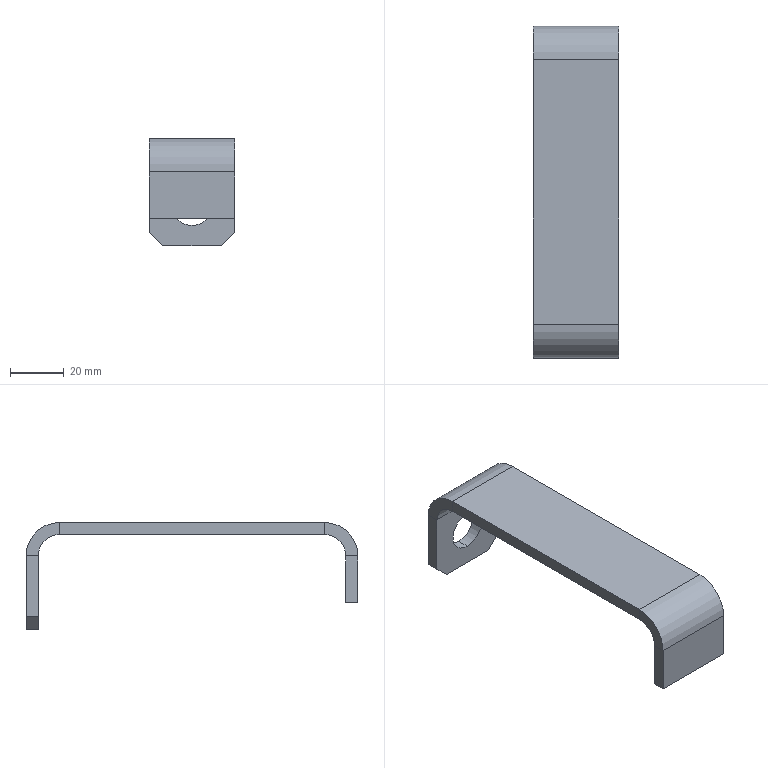Part | SolidWorks | features Chamfer 1, FlatPattern 1, ICE 1, SMBaseFlange 1, SheetMetal 1 | 1 solid | 26 faces | box 32 x 124 x 40 mm | volume 24465 mm3 | plane 20 | cylinder 6 | commonest cylinder face diameters 15 x2 16 x2 25 x2
STEP:
#1=CARTESIAN_POINT('',(0.,119.5,12.5));
#2=VERTEX_POINT('',#1);
#3=CARTESIAN_POINT('',(0.,119.5,-2.5));
#4=VERTEX_POINT('',#3);
#5=CARTESIAN_POINT('',(0.,119.5,5.));
#6=DIRECTION('',(0.,-1.,0.));
#7=DIRECTION('',(0.,0.,1.));
#8=AXIS2_PLACEMENT_3D('',#5,#6,#7);
#9=CIRCLE('',#8,7.5);
#10=EDGE_CURVE('',#2,#4,#9,.T.);
#11=ORIENTED_EDGE('',*,*,#10,.T.);
#12=CARTESIAN_POINT('',(0.,124.,-2.5));
#13=VERTEX_POINT('',#12);
#14=CARTESIAN_POINT('',(0.,-0.001,-2.5));
#15=DIRECTION('',(0.,1.,0.));
#16=VECTOR('',#15,1000.);
#17=LINE('',#14,#16);
#18=EDGE_CURVE('',#4,#13,#17,.T.);
#19=ORIENTED_EDGE('',*,*,#18,.T.);
#20=CARTESIAN_POINT('',(0.,124.,12.5));
#21=VERTEX_POINT('',#20);
#22=CARTESIAN_POINT('',(0.,124.,5.));
#23=DIRECTION('',(0.,1.,0.));
#24=DIRECTION('',(0.,0.,1.));
#25=AXIS2_PLACEMENT_3D('',#22,#23,#24);
#26=CIRCLE('',#25,7.5);
#27=EDGE_CURVE('',#13,#21,#26,.T.);
#28=ORIENTED_EDGE('',*,*,#27,.T.);
#29=CARTESIAN_POINT('',(0.,-0.001,12.5));
#30=DIRECTION('',(0.,1.,0.));
#31=VECTOR('',#30,1000.);
#32=LINE('',#29,#31);
#33=EDGE_CURVE('',#2,#21,#32,.T.);
#34=ORIENTED_EDGE('',*,*,#33,.F.);
#35=EDGE_LOOP('',(#11,#19,#28,#34));
#36=FACE_OUTER_BOUND('',#35,.T.);
#37=CARTESIAN_POINT('',(0.,-0.001,5.));
#38=DIRECTION('',(0.,1.,0.));
#39=DIRECTION('',(0.,0.,1.));
#40=AXIS2_PLACEMENT_3D('',#37,#38,#39);
#41=CYLINDRICAL_SURFACE('',#40,7.5);
#42=ADVANCED_FACE('',(#36),#41,.F.);
#43=CARTESIAN_POINT('',(16.,12.5,30.));
#44=VERTEX_POINT('',#43);
#45=CARTESIAN_POINT('',(16.,12.5,25.5));
#46=VERTEX_POINT('',#45);
#47=CARTESIAN_POINT('',(16.,12.5,30.));
#48=DIRECTION('',(0.,0.,-1.));
#49=VECTOR('',#48,1000.);
#50=LINE('',#47,#49);
#51=EDGE_CURVE('',#44,#46,#50,.T.);
#52=ORIENTED_EDGE('',*,*,#51,.F.);
#53=CARTESIAN_POINT('',(16.,0.,17.5));
#54=VERTEX_POINT('',#53);
#55=CARTESIAN_POINT('',(16.,12.5,17.5));
#56=DIRECTION('',(-1.,0.,0.));
#57=DIRECTION('',(0.,0.,-1.));
#58=AXIS2_PLACEMENT_3D('',#55,#56,#57);
#59=CIRCLE('',#58,12.5);
#60=EDGE_CURVE('',#54,#44,#59,.T.);
#61=ORIENTED_EDGE('',*,*,#60,.F.);
#62=CARTESIAN_POINT('',(16.,4.5,17.5));
#63=VERTEX_POINT('',#62);
#64=CARTESIAN_POINT('',(16.,4.5,17.5));
#65=DIRECTION('',(0.,-1.,0.));
#66=VECTOR('',#65,1000.);
#67=LINE('',#64,#66);
#68=EDGE_CURVE('',#63,#54,#67,.T.);
#69=ORIENTED_EDGE('',*,*,#68,.F.);
#70=CARTESIAN_POINT('',(16.,12.5,17.5));
#71=DIRECTION('',(-1.,0.,0.));
#72=DIRECTION('',(0.,0.,-1.));
#73=AXIS2_PLACEMENT_3D('',#70,#71,#72);
#74=CIRCLE('',#73,8.);
#75=EDGE_CURVE('',#63,#46,#74,.T.);
#76=ORIENTED_EDGE('',*,*,#75,.T.);
#77=EDGE_LOOP('',(#52,#61,#69,#76));
#78=FACE_OUTER_BOUND('',#77,.T.);
#79=CARTESIAN_POINT('',(16.,12.5,30.));
#80=DIRECTION('',(1.,0.,0.));
#81=DIRECTION('',(0.,0.,-1.));
#82=AXIS2_PLACEMENT_3D('',#79,#80,#81);
#83=PLANE('',#82);
#84=ADVANCED_FACE('',(#78),#83,.T.);
#85=CARTESIAN_POINT('',(16.,111.5,30.));
#86=VERTEX_POINT('',#85);
#87=CARTESIAN_POINT('',(16.,0.,30.));
#88=DIRECTION('',(0.,1.,0.));
#89=VECTOR('',#88,1000.);
#90=LINE('',#87,#89);
#91=EDGE_CURVE('',#44,#86,#90,.T.);
#92=ORIENTED_EDGE('',*,*,#91,.F.);
#93=ORIENTED_EDGE('',*,*,#51,.T.);
#94=CARTESIAN_POINT('',(16.,111.5,25.5));
#95=VERTEX_POINT('',#94);
#96=CARTESIAN_POINT('',(16.,0.,25.5));
#97=DIRECTION('',(0.,1.,0.));
#98=VECTOR('',#97,1000.);
#99=LINE('',#96,#98);
#100=EDGE_CURVE('',#46,#95,#99,.T.);
#101=ORIENTED_EDGE('',*,*,#100,.T.);
#102=CARTESIAN_POINT('',(16.,111.5,25.5));
#103=DIRECTION('',(0.,0.,1.));
#104=VECTOR('',#103,1000.);
#105=LINE('',#102,#104);
#106=EDGE_CURVE('',#95,#86,#105,.T.);
#107=ORIENTED_EDGE('',*,*,#106,.T.);
#108=EDGE_LOOP('',(#92,#93,#101,#107));
#109=FACE_OUTER_BOUND('',#108,.T.);
#110=CARTESIAN_POINT('',(16.,4.5,17.5));
#111=DIRECTION('',(1.,0.,0.));
#112=DIRECTION('',(0.,0.,-1.));
#113=AXIS2_PLACEMENT_3D('',#110,#111,#112);
#114=PLANE('',#113);
#115=ADVANCED_FACE('',(#109),#114,.T.);
#116=CARTESIAN_POINT('',(-16.,0.,17.5));
#117=VERTEX_POINT('',#116);
#118=CARTESIAN_POINT('',(-16.,4.5,17.5));
#119=VERTEX_POINT('',#118);
#120=CARTESIAN_POINT('',(-16.,0.,17.5));
#121=DIRECTION('',(0.,1.,0.));
#122=VECTOR('',#121,1000.);
#123=LINE('',#120,#122);
#124=EDGE_CURVE('',#117,#119,#123,.T.);
#125=ORIENTED_EDGE('',*,*,#124,.F.);
#126=CARTESIAN_POINT('',(-16.,12.5,30.));
#127=VERTEX_POINT('',#126);
#128=CARTESIAN_POINT('',(-16.,12.5,17.5));
#129=DIRECTION('',(-1.,0.,0.));
#130=DIRECTION('',(0.,0.,-1.));
#131=AXIS2_PLACEMENT_3D('',#128,#129,#130);
#132=CIRCLE('',#131,12.5);
#133=EDGE_CURVE('',#117,#127,#132,.T.);
#134=ORIENTED_EDGE('',*,*,#133,.T.);
#135=CARTESIAN_POINT('',(-16.,12.5,25.5));
#136=VERTEX_POINT('',#135);
#137=CARTESIAN_POINT('',(-16.,12.5,25.5));
#138=DIRECTION('',(0.,0.,1.));
#139=VECTOR('',#138,1000.);
#140=LINE('',#137,#139);
#141=EDGE_CURVE('',#136,#127,#140,.T.);
#142=ORIENTED_EDGE('',*,*,#141,.F.);
#143=CARTESIAN_POINT('',(-16.,12.5,17.5));
#144=DIRECTION('',(-1.,0.,0.));
#145=DIRECTION('',(0.,0.,-1.));
#146=AXIS2_PLACEMENT_3D('',#143,#144,#145);
#147=CIRCLE('',#146,8.);
#148=EDGE_CURVE('',#119,#136,#147,.T.);
#149=ORIENTED_EDGE('',*,*,#148,.F.);
#150=EDGE_LOOP('',(#125,#134,#142,#149));
#151=FACE_OUTER_BOUND('',#150,.T.);
#152=CARTESIAN_POINT('',(-16.,0.,17.5));
#153=DIRECTION('',(-1.,0.,0.));
#154=DIRECTION('',(0.,0.,1.));
#155=AXIS2_PLACEMENT_3D('',#152,#153,#154);
#156=PLANE('',#155);
#157=ADVANCED_FACE('',(#151),#156,.T.);
#158=CARTESIAN_POINT('',(-16.,0.,0.));
#159=VERTEX_POINT('',#158);
#160=CARTESIAN_POINT('',(-16.,0.,0.));
#161=DIRECTION('',(0.,0.,1.));
#162=VECTOR('',#161,1000.);
#163=LINE('',#160,#162);
#164=EDGE_CURVE('',#159,#117,#163,.T.);
#165=ORIENTED_EDGE('',*,*,#164,.T.);
#166=ORIENTED_EDGE('',*,*,#124,.T.);
#167=CARTESIAN_POINT('',(-16.,4.5,0.));
#168=VERTEX_POINT('',#167);
#169=CARTESIAN_POINT('',(-16.,4.5,0.));
#170=DIRECTION('',(0.,0.,1.));
#171=VECTOR('',#170,1000.);
#172=LINE('',#169,#171);
#173=EDGE_CURVE('',#168,#119,#172,.T.);
#174=ORIENTED_EDGE('',*,*,#173,.F.);
#175=CARTESIAN_POINT('',(-16.,4.5,0.));
#176=DIRECTION('',(0.,-1.,0.));
#177=VECTOR('',#176,1000.);
#178=LINE('',#175,#177);
#179=EDGE_CURVE('',#168,#159,#178,.T.);
#180=ORIENTED_EDGE('',*,*,#179,.T.);
#181=EDGE_LOOP('',(#165,#166,#174,#180));
#182=FACE_OUTER_BOUND('',#181,.T.);
#183=CARTESIAN_POINT('',(-16.,12.5,25.5));
#184=DIRECTION('',(-1.,0.,0.));
#185=DIRECTION('',(0.,0.,1.));
#186=AXIS2_PLACEMENT_3D('',#183,#184,#185);
#187=PLANE('',#186);
#188=ADVANCED_FACE('',(#182),#187,.T.);
#189=CARTESIAN_POINT('',(16.,124.,17.5));
#190=VERTEX_POINT('',#189);
#191=CARTESIAN_POINT('',(16.,119.5,17.5));
#192=VERTEX_POINT('',#191);
#193=CARTESIAN_POINT('',(16.,124.,17.5));
#194=DIRECTION('',(0.,-1.,0.));
#195=VECTOR('',#194,1000.);
#196=LINE('',#193,#195);
#197=EDGE_CURVE('',#190,#192,#196,.T.);
#198=ORIENTED_EDGE('',*,*,#197,.F.);
#199=CARTESIAN_POINT('',(16.,111.5,17.5));
#200=DIRECTION('',(-1.,0.,0.));
#201=DIRECTION('',(0.,0.,-1.));
#202=AXIS2_PLACEMENT_3D('',#199,#200,#201);
#203=CIRCLE('',#202,12.5);
#204=EDGE_CURVE('',#86,#190,#203,.T.);
#205=ORIENTED_EDGE('',*,*,#204,.F.);
#206=ORIENTED_EDGE('',*,*,#106,.F.);
#207=CARTESIAN_POINT('',(16.,111.5,17.5));
#208=DIRECTION('',(-1.,0.,0.));
#209=DIRECTION('',(0.,0.,-1.));
#210=AXIS2_PLACEMENT_3D('',#207,#208,#209);
#211=CIRCLE('',#210,8.);
#212=EDGE_CURVE('',#95,#192,#211,.T.);
#213=ORIENTED_EDGE('',*,*,#212,.T.);
#214=EDGE_LOOP('',(#198,#205,#206,#213));
#215=FACE_OUTER_BOUND('',#214,.T.);
#216=CARTESIAN_POINT('',(16.,124.,17.5));
#217=DIRECTION('',(1.,0.,0.));
#218=DIRECTION('',(0.,0.,-1.));
#219=AXIS2_PLACEMENT_3D('',#216,#217,#218);
#220=PLANE('',#219);
#221=ADVANCED_FACE('',(#215),#220,.T.);
#222=CARTESIAN_POINT('',(16.,119.5,-5.));
#223=VERTEX_POINT('',#222);
#224=CARTESIAN_POINT('',(16.,119.5,30.));
#225=DIRECTION('',(0.,0.,-1.));
#226=VECTOR('',#225,1000.);
#227=LINE('',#224,#226);
#228=EDGE_CURVE('',#192,#223,#227,.T.);
#229=ORIENTED_EDGE('',*,*,#228,.T.);
#230=CARTESIAN_POINT('',(16.,124.,-5.));
#231=VERTEX_POINT('',#230);
#232=CARTESIAN_POINT('',(16.,111.5,-5.));
#233=DIRECTION('',(0.,1.,0.));
#234=VECTOR('',#233,1000.);
#235=LINE('',#232,#234);
#236=EDGE_CURVE('',#223,#231,#235,.T.);
#237=ORIENTED_EDGE('',*,*,#236,.T.);
#238=CARTESIAN_POINT('',(16.,124.,30.));
#239=DIRECTION('',(0.,0.,-1.));
#240=VECTOR('',#239,1000.);
#241=LINE('',#238,#240);
#242=EDGE_CURVE('',#190,#231,#241,.T.);
#243=ORIENTED_EDGE('',*,*,#242,.F.);
#244=ORIENTED_EDGE('',*,*,#197,.T.);
#245=EDGE_LOOP('',(#229,#237,#243,#244));
#246=FACE_OUTER_BOUND('',#245,.T.);
#247=CARTESIAN_POINT('',(16.,111.5,25.5));
#248=DIRECTION('',(1.,0.,0.));
#249=DIRECTION('',(0.,0.,-1.));
#250=AXIS2_PLACEMENT_3D('',#247,#248,#249);
#251=PLANE('',#250);
#252=ADVANCED_FACE('',(#246),#251,.T.);
#253=CARTESIAN_POINT('',(-16.,111.5,30.));
#254=VERTEX_POINT('',#253);
#255=CARTESIAN_POINT('',(-16.,111.5,25.5));
#256=VERTEX_POINT('',#255);
#257=CARTESIAN_POINT('',(-16.,111.5,30.));
#258=DIRECTION('',(0.,0.,-1.));
#259=VECTOR('',#258,1000.);
#260=LINE('',#257,#259);
#261=EDGE_CURVE('',#254,#256,#260,.T.);
#262=ORIENTED_EDGE('',*,*,#261,.F.);
#263=CARTESIAN_POINT('',(-16.,124.,17.5));
#264=VERTEX_POINT('',#263);
#265=CARTESIAN_POINT('',(-16.,111.5,17.5));
#266=DIRECTION('',(-1.,0.,0.));
#267=DIRECTION('',(0.,0.,-1.));
#268=AXIS2_PLACEMENT_3D('',#265,#266,#267);
#269=CIRCLE('',#268,12.5);
#270=EDGE_CURVE('',#254,#264,#269,.T.);
#271=ORIENTED_EDGE('',*,*,#270,.T.);
#272=CARTESIAN_POINT('',(-16.,119.5,17.5));
#273=VERTEX_POINT('',#272);
#274=CARTESIAN_POINT('',(-16.,119.5,17.5));
#275=DIRECTION('',(0.,1.,0.));
#276=VECTOR('',#275,1000.);
#277=LINE('',#274,#276);
#278=EDGE_CURVE('',#273,#264,#277,.T.);
#279=ORIENTED_EDGE('',*,*,#278,.F.);
#280=CARTESIAN_POINT('',(-16.,111.5,17.5));
#281=DIRECTION('',(-1.,0.,0.));
#282=DIRECTION('',(0.,0.,-1.));
#283=AXIS2_PLACEMENT_3D('',#280,#281,#282);
#284=CIRCLE('',#283,8.);
#285=EDGE_CURVE('',#256,#273,#284,.T.);
#286=ORIENTED_EDGE('',*,*,#285,.F.);
#287=EDGE_LOOP('',(#262,#271,#279,#286));
#288=FACE_OUTER_BOUND('',#287,.T.);
#289=CARTESIAN_POINT('',(-16.,111.5,30.));
#290=DIRECTION('',(-1.,0.,0.));
#291=DIRECTION('',(0.,0.,1.));
#292=AXIS2_PLACEMENT_3D('',#289,#290,#291);
#293=PLANE('',#292);
#294=ADVANCED_FACE('',(#288),#293,.T.);
#295=CARTESIAN_POINT('',(-16.,0.,30.));
#296=DIRECTION('',(0.,1.,0.));
#297=VECTOR('',#296,1000.);
#298=LINE('',#295,#297);
#299=EDGE_CURVE('',#127,#254,#298,.T.);
#300=ORIENTED_EDGE('',*,*,#299,.T.);
#301=ORIENTED_EDGE('',*,*,#261,.T.);
#302=CARTESIAN_POINT('',(-16.,0.,25.5));
#303=DIRECTION('',(0.,1.,0.));
#304=VECTOR('',#303,1000.);
#305=LINE('',#302,#304);
#306=EDGE_CURVE('',#136,#256,#305,.T.);
#307=ORIENTED_EDGE('',*,*,#306,.F.);
#308=ORIENTED_EDGE('',*,*,#141,.T.);
#309=EDGE_LOOP('',(#300,#301,#307,#308));
#310=FACE_OUTER_BOUND('',#309,.T.);
#311=CARTESIAN_POINT('',(-16.,119.5,17.5));
#312=DIRECTION('',(-1.,0.,0.));
#313=DIRECTION('',(0.,0.,1.));
#314=AXIS2_PLACEMENT_3D('',#311,#312,#313);
#315=PLANE('',#314);
#316=ADVANCED_FACE('',(#310),#315,.T.);
#317=ORIENTED_EDGE('',*,*,#10,.F.);
#318=CARTESIAN_POINT('',(0.,119.5,5.));
#319=DIRECTION('',(0.,-1.,0.));
#320=DIRECTION('',(0.,0.,1.));
#321=AXIS2_PLACEMENT_3D('',#318,#319,#320);
#322=CIRCLE('',#321,7.5);
#323=EDGE_CURVE('',#4,#2,#322,.T.);
#324=ORIENTED_EDGE('',*,*,#323,.F.);
#325=EDGE_LOOP('',(#317,#324));
#326=FACE_BOUND('',#325,.T.);
#327=CARTESIAN_POINT('',(-16.,119.5,-5.));
#328=VERTEX_POINT('',#327);
#329=CARTESIAN_POINT('',(-16.,119.5,30.));
#330=DIRECTION('',(0.,0.,-1.));
#331=VECTOR('',#330,1000.);
#332=LINE('',#329,#331);
#333=EDGE_CURVE('',#273,#328,#332,.T.);
#334=ORIENTED_EDGE('',*,*,#333,.T.);
#335=CARTESIAN_POINT('',(-11.,119.5,-10.));
#336=VERTEX_POINT('',#335);
#337=CARTESIAN_POINT('',(-16.,119.5,-5.));
#338=DIRECTION('',(0.7071,0.,-0.7071));
#339=VECTOR('',#338,1000.);
#340=LINE('',#337,#339);
#341=EDGE_CURVE('',#328,#336,#340,.T.);
#342=ORIENTED_EDGE('',*,*,#341,.T.);
#343=CARTESIAN_POINT('',(11.,119.5,-10.));
#344=VERTEX_POINT('',#343);
#345=CARTESIAN_POINT('',(16.,119.5,-10.));
#346=DIRECTION('',(-1.,0.,0.));
#347=VECTOR('',#346,1000.);
#348=LINE('',#345,#347);
#349=EDGE_CURVE('',#344,#336,#348,.T.);
#350=ORIENTED_EDGE('',*,*,#349,.F.);
#351=CARTESIAN_POINT('',(11.,119.5,-10.));
#352=DIRECTION('',(0.7071,0.,0.7071));
#353=VECTOR('',#352,1000.);
#354=LINE('',#351,#353);
#355=EDGE_CURVE('',#344,#223,#354,.T.);
#356=ORIENTED_EDGE('',*,*,#355,.T.);
#357=ORIENTED_EDGE('',*,*,#228,.F.);
#358=CARTESIAN_POINT('',(16.,119.5,17.5));
#359=DIRECTION('',(-1.,0.,0.));
#360=VECTOR('',#359,1000.);
#361=LINE('',#358,#360);
#362=EDGE_CURVE('',#192,#273,#361,.T.);
#363=ORIENTED_EDGE('',*,*,#362,.T.);
#364=EDGE_LOOP('',(#334,#342,#350,#356,#357,#363));
#365=FACE_OUTER_BOUND('',#364,.T.);
#366=CARTESIAN_POINT('',(16.,119.5,30.));
#367=DIRECTION('',(0.,1.,0.));
#368=DIRECTION('',(0.,0.,1.));
#369=AXIS2_PLACEMENT_3D('',#366,#367,#368);
#370=PLANE('',#369);
#371=ADVANCED_FACE('',(#326,#365),#370,.F.);
#372=ORIENTED_EDGE('',*,*,#349,.T.);
#373=CARTESIAN_POINT('',(-11.,124.,-10.));
#374=VERTEX_POINT('',#373);
#375=CARTESIAN_POINT('',(-11.,124.,-10.));
#376=DIRECTION('',(0.,1.,0.));
#377=VECTOR('',#376,1000.);
#378=LINE('',#375,#377);
#379=EDGE_CURVE('',#336,#374,#378,.T.);
#380=ORIENTED_EDGE('',*,*,#379,.T.);
#381=CARTESIAN_POINT('',(11.,124.,-10.));
#382=VERTEX_POINT('',#381);
#383=CARTESIAN_POINT('',(16.,124.,-10.));
#384=DIRECTION('',(-1.,0.,0.));
#385=VECTOR('',#384,1000.);
#386=LINE('',#383,#385);
#387=EDGE_CURVE('',#382,#374,#386,.T.);
#388=ORIENTED_EDGE('',*,*,#387,.F.);
#389=CARTESIAN_POINT('',(11.,124.,-10.));
#390=DIRECTION('',(0.,-1.,0.));
#391=VECTOR('',#390,1000.);
#392=LINE('',#389,#391);
#393=EDGE_CURVE('',#382,#344,#392,.T.);
#394=ORIENTED_EDGE('',*,*,#393,.T.);
#395=EDGE_LOOP('',(#372,#380,#388,#394));
#396=FACE_OUTER_BOUND('',#395,.T.);
#397=CARTESIAN_POINT('',(16.,124.,-10.));
#398=DIRECTION('',(0.,0.,-1.));
#399=DIRECTION('',(-1.,0.,0.));
#400=AXIS2_PLACEMENT_3D('',#397,#398,#399);
#401=PLANE('',#400);
#402=ADVANCED_FACE('',(#396),#401,.T.);
#403=CARTESIAN_POINT('',(0.,124.,5.));
#404=DIRECTION('',(0.,1.,0.));
#405=DIRECTION('',(0.,0.,1.));
#406=AXIS2_PLACEMENT_3D('',#403,#404,#405);
#407=CIRCLE('',#406,7.5);
#408=EDGE_CURVE('',#21,#13,#407,.T.);
#409=ORIENTED_EDGE('',*,*,#408,.F.);
#410=ORIENTED_EDGE('',*,*,#27,.F.);
#411=EDGE_LOOP('',(#409,#410));
#412=FACE_BOUND('',#411,.T.);
#413=ORIENTED_EDGE('',*,*,#387,.T.);
#414=CARTESIAN_POINT('',(-16.,124.,-5.));
#415=VERTEX_POINT('',#414);
#416=CARTESIAN_POINT('',(-17.5,124.,-3.5));
#417=DIRECTION('',(-0.7071,0.,0.7071));
#418=VECTOR('',#417,1000.);
#419=LINE('',#416,#418);
#420=EDGE_CURVE('',#374,#415,#419,.T.);
#421=ORIENTED_EDGE('',*,*,#420,.T.);
#422=CARTESIAN_POINT('',(-16.,124.,30.));
#423=DIRECTION('',(0.,0.,-1.));
#424=VECTOR('',#423,1000.);
#425=LINE('',#422,#424);
#426=EDGE_CURVE('',#264,#415,#425,.T.);
#427=ORIENTED_EDGE('',*,*,#426,.F.);
#428=CARTESIAN_POINT('',(16.,124.,17.5));
#429=DIRECTION('',(-1.,0.,0.));
#430=VECTOR('',#429,1000.);
#431=LINE('',#428,#430);
#432=EDGE_CURVE('',#190,#264,#431,.T.);
#433=ORIENTED_EDGE('',*,*,#432,.F.);
#434=ORIENTED_EDGE('',*,*,#242,.T.);
#435=CARTESIAN_POINT('',(33.5,124.,12.5));
#436=DIRECTION('',(-0.7071,0.,-0.7071));
#437=VECTOR('',#436,1000.);
#438=LINE('',#435,#437);
#439=EDGE_CURVE('',#231,#382,#438,.T.);
#440=ORIENTED_EDGE('',*,*,#439,.T.);
#441=EDGE_LOOP('',(#413,#421,#427,#433,#434,#440));
#442=FACE_OUTER_BOUND('',#441,.T.);
#443=CARTESIAN_POINT('',(16.,124.,30.));
#444=DIRECTION('',(0.,1.,0.));
#445=DIRECTION('',(0.,0.,1.));
#446=AXIS2_PLACEMENT_3D('',#443,#444,#445);
#447=PLANE('',#446);
#448=ADVANCED_FACE('',(#412,#442),#447,.T.);
#449=ORIENTED_EDGE('',*,*,#270,.F.);
#450=CARTESIAN_POINT('',(16.,111.5,30.));
#451=DIRECTION('',(-1.,0.,0.));
#452=VECTOR('',#451,1000.);
#453=LINE('',#450,#452);
#454=EDGE_CURVE('',#86,#254,#453,.T.);
#455=ORIENTED_EDGE('',*,*,#454,.F.);
#456=ORIENTED_EDGE('',*,*,#204,.T.);
#457=ORIENTED_EDGE('',*,*,#432,.T.);
#458=EDGE_LOOP('',(#449,#455,#456,#457));
#459=FACE_OUTER_BOUND('',#458,.T.);
#460=CARTESIAN_POINT('',(16.,111.5,17.5));
#461=DIRECTION('',(-1.,0.,0.));
#462=DIRECTION('',(0.,0.,1.));
#463=AXIS2_PLACEMENT_3D('',#460,#461,#462);
#464=CYLINDRICAL_SURFACE('',#463,12.5);
#465=ADVANCED_FACE('',(#459),#464,.T.);
#466=ORIENTED_EDGE('',*,*,#299,.F.);
#467=CARTESIAN_POINT('',(16.,12.5,30.));
#468=DIRECTION('',(-1.,0.,0.));
#469=VECTOR('',#468,1000.);
#470=LINE('',#467,#469);
#471=EDGE_CURVE('',#44,#127,#470,.T.);
#472=ORIENTED_EDGE('',*,*,#471,.F.);
#473=ORIENTED_EDGE('',*,*,#91,.T.);
#474=ORIENTED_EDGE('',*,*,#454,.T.);
#475=EDGE_LOOP('',(#466,#472,#473,#474));
#476=FACE_OUTER_BOUND('',#475,.T.);
#477=CARTESIAN_POINT('',(16.,0.,30.));
#478=DIRECTION('',(0.,0.,1.));
#479=DIRECTION('',(1.,0.,0.));
#480=AXIS2_PLACEMENT_3D('',#477,#478,#479);
#481=PLANE('',#480);
#482=ADVANCED_FACE('',(#476),#481,.T.);
#483=ORIENTED_EDGE('',*,*,#133,.F.);
#484=CARTESIAN_POINT('',(16.,0.,17.5));
#485=DIRECTION('',(-1.,0.,0.));
#486=VECTOR('',#485,1000.);
#487=LINE('',#484,#486);
#488=EDGE_CURVE('',#54,#117,#487,.T.);
#489=ORIENTED_EDGE('',*,*,#488,.F.);
#490=ORIENTED_EDGE('',*,*,#60,.T.);
#491=ORIENTED_EDGE('',*,*,#471,.T.);
#492=EDGE_LOOP('',(#483,#489,#490,#491));
#493=FACE_OUTER_BOUND('',#492,.T.);
#494=CARTESIAN_POINT('',(16.,12.5,17.5));
#495=DIRECTION('',(-1.,0.,0.));
#496=DIRECTION('',(0.,0.,1.));
#497=AXIS2_PLACEMENT_3D('',#494,#495,#496);
#498=CYLINDRICAL_SURFACE('',#497,12.5);
#499=ADVANCED_FACE('',(#493),#498,.T.);
#500=ORIENTED_EDGE('',*,*,#164,.F.);
#501=CARTESIAN_POINT('',(16.,0.,0.));
#502=VERTEX_POINT('',#501);
#503=CARTESIAN_POINT('',(16.,0.,0.));
#504=DIRECTION('',(-1.,0.,0.));
#505=VECTOR('',#504,1000.);
#506=LINE('',#503,#505);
#507=EDGE_CURVE('',#502,#159,#506,.T.);
#508=ORIENTED_EDGE('',*,*,#507,.F.);
#509=CARTESIAN_POINT('',(16.,0.,0.));
#510=DIRECTION('',(0.,0.,1.));
#511=VECTOR('',#510,1000.);
#512=LINE('',#509,#511);
#513=EDGE_CURVE('',#502,#54,#512,.T.);
#514=ORIENTED_EDGE('',*,*,#513,.T.);
#515=ORIENTED_EDGE('',*,*,#488,.T.);
#516=EDGE_LOOP('',(#500,#508,#514,#515));
#517=FACE_OUTER_BOUND('',#516,.T.);
#518=CARTESIAN_POINT('',(16.,0.,0.));
#519=DIRECTION('',(0.,-1.,0.));
#520=DIRECTION('',(0.,0.,-1.));
#521=AXIS2_PLACEMENT_3D('',#518,#519,#520);
#522=PLANE('',#521);
#523=ADVANCED_FACE('',(#517),#522,.T.);
#524=ORIENTED_EDGE('',*,*,#179,.F.);
#525=CARTESIAN_POINT('',(16.,4.5,0.));
#526=VERTEX_POINT('',#525);
#527=CARTESIAN_POINT('',(16.,4.5,0.));
#528=DIRECTION('',(-1.,0.,0.));
#529=VECTOR('',#528,1000.);
#530=LINE('',#527,#529);
#531=EDGE_CURVE('',#526,#168,#530,.T.);
#532=ORIENTED_EDGE('',*,*,#531,.F.);
#533=CARTESIAN_POINT('',(16.,4.5,0.));
#534=DIRECTION('',(0.,-1.,0.));
#535=VECTOR('',#534,1000.);
#536=LINE('',#533,#535);
#537=EDGE_CURVE('',#526,#502,#536,.T.);
#538=ORIENTED_EDGE('',*,*,#537,.T.);
#539=ORIENTED_EDGE('',*,*,#507,.T.);
#540=EDGE_LOOP('',(#524,#532,#538,#539));
#541=FACE_OUTER_BOUND('',#540,.T.);
#542=CARTESIAN_POINT('',(16.,4.5,0.));
#543=DIRECTION('',(0.,0.,-1.));
#544=DIRECTION('',(-1.,0.,0.));
#545=AXIS2_PLACEMENT_3D('',#542,#543,#544);
#546=PLANE('',#545);
#547=ADVANCED_FACE('',(#541),#546,.T.);
#548=ORIENTED_EDGE('',*,*,#173,.T.);
#549=CARTESIAN_POINT('',(16.,4.5,17.5));
#550=DIRECTION('',(-1.,0.,0.));
#551=VECTOR('',#550,1000.);
#552=LINE('',#549,#551);
#553=EDGE_CURVE('',#63,#119,#552,.T.);
#554=ORIENTED_EDGE('',*,*,#553,.F.);
#555=CARTESIAN_POINT('',(16.,4.5,0.));
#556=DIRECTION('',(0.,0.,1.));
#557=VECTOR('',#556,1000.);
#558=LINE('',#555,#557);
#559=EDGE_CURVE('',#526,#63,#558,.T.);
#560=ORIENTED_EDGE('',*,*,#559,.F.);
#561=ORIENTED_EDGE('',*,*,#531,.T.);
#562=EDGE_LOOP('',(#548,#554,#560,#561));
#563=FACE_OUTER_BOUND('',#562,.T.);
#564=CARTESIAN_POINT('',(16.,4.5,0.));
#565=DIRECTION('',(0.,-1.,0.));
#566=DIRECTION('',(0.,0.,-1.));
#567=AXIS2_PLACEMENT_3D('',#564,#565,#566);
#568=PLANE('',#567);
#569=ADVANCED_FACE('',(#563),#568,.F.);
#570=ORIENTED_EDGE('',*,*,#148,.T.);
#571=CARTESIAN_POINT('',(16.,12.5,25.5));
#572=DIRECTION('',(-1.,0.,0.));
#573=VECTOR('',#572,1000.);
#574=LINE('',#571,#573);
#575=EDGE_CURVE('',#46,#136,#574,.T.);
#576=ORIENTED_EDGE('',*,*,#575,.F.);
#577=ORIENTED_EDGE('',*,*,#75,.F.);
#578=ORIENTED_EDGE('',*,*,#553,.T.);
#579=EDGE_LOOP('',(#570,#576,#577,#578));
#580=FACE_OUTER_BOUND('',#579,.T.);
#581=CARTESIAN_POINT('',(16.,12.5,17.5));
#582=DIRECTION('',(-1.,0.,0.));
#583=DIRECTION('',(0.,0.,1.));
#584=AXIS2_PLACEMENT_3D('',#581,#582,#583);
#585=CYLINDRICAL_SURFACE('',#584,8.);
#586=ADVANCED_FACE('',(#580),#585,.F.);
#587=ORIENTED_EDGE('',*,*,#306,.T.);
#588=CARTESIAN_POINT('',(16.,111.5,25.5));
#589=DIRECTION('',(-1.,0.,0.));
#590=VECTOR('',#589,1000.);
#591=LINE('',#588,#590);
#592=EDGE_CURVE('',#95,#256,#591,.T.);
#593=ORIENTED_EDGE('',*,*,#592,.F.);
#594=ORIENTED_EDGE('',*,*,#100,.F.);
#595=ORIENTED_EDGE('',*,*,#575,.T.);
#596=EDGE_LOOP('',(#587,#593,#594,#595));
#597=FACE_OUTER_BOUND('',#596,.T.);
#598=CARTESIAN_POINT('',(16.,0.,25.5));
#599=DIRECTION('',(0.,0.,1.));
#600=DIRECTION('',(1.,0.,0.));
#601=AXIS2_PLACEMENT_3D('',#598,#599,#600);
#602=PLANE('',#601);
#603=ADVANCED_FACE('',(#597),#602,.F.);
#604=ORIENTED_EDGE('',*,*,#285,.T.);
#605=ORIENTED_EDGE('',*,*,#362,.F.);
#606=ORIENTED_EDGE('',*,*,#212,.F.);
#607=ORIENTED_EDGE('',*,*,#592,.T.);
#608=EDGE_LOOP('',(#604,#605,#606,#607));
#609=FACE_OUTER_BOUND('',#608,.T.);
#610=CARTESIAN_POINT('',(16.,111.5,17.5));
#611=DIRECTION('',(-1.,0.,0.));
#612=DIRECTION('',(0.,0.,1.));
#613=AXIS2_PLACEMENT_3D('',#610,#611,#612);
#614=CYLINDRICAL_SURFACE('',#613,8.);
#615=ADVANCED_FACE('',(#609),#614,.F.);
#616=ORIENTED_EDGE('',*,*,#559,.T.);
#617=ORIENTED_EDGE('',*,*,#68,.T.);
#618=ORIENTED_EDGE('',*,*,#513,.F.);
#619=ORIENTED_EDGE('',*,*,#537,.F.);
#620=EDGE_LOOP('',(#616,#617,#618,#619));
#621=FACE_OUTER_BOUND('',#620,.T.);
#622=CARTESIAN_POINT('',(16.,111.5,17.5));
#623=DIRECTION('',(1.,0.,0.));
#624=DIRECTION('',(0.,0.,-1.));
#625=AXIS2_PLACEMENT_3D('',#622,#623,#624);
#626=PLANE('',#625);
#627=ADVANCED_FACE('',(#621),#626,.T.);
#628=ORIENTED_EDGE('',*,*,#426,.T.);
#629=CARTESIAN_POINT('',(-16.,119.5,-5.));
#630=DIRECTION('',(0.,-1.,0.));
#631=VECTOR('',#630,1000.);
#632=LINE('',#629,#631);
#633=EDGE_CURVE('',#415,#328,#632,.T.);
#634=ORIENTED_EDGE('',*,*,#633,.T.);
#635=ORIENTED_EDGE('',*,*,#333,.F.);
#636=ORIENTED_EDGE('',*,*,#278,.T.);
#637=EDGE_LOOP('',(#628,#634,#635,#636));
#638=FACE_OUTER_BOUND('',#637,.T.);
#639=CARTESIAN_POINT('',(-16.,111.5,17.5));
#640=DIRECTION('',(1.,0.,0.));
#641=DIRECTION('',(0.,0.,-1.));
#642=AXIS2_PLACEMENT_3D('',#639,#640,#641);
#643=PLANE('',#642);
#644=ADVANCED_FACE('',(#638),#643,.F.);
#645=ORIENTED_EDGE('',*,*,#18,.F.);
#646=ORIENTED_EDGE('',*,*,#323,.T.);
#647=ORIENTED_EDGE('',*,*,#33,.T.);
#648=ORIENTED_EDGE('',*,*,#408,.T.);
#649=EDGE_LOOP('',(#645,#646,#647,#648));
#650=FACE_OUTER_BOUND('',#649,.T.);
#651=CARTESIAN_POINT('',(0.,-0.001,5.));
#652=DIRECTION('',(0.,1.,0.));
#653=DIRECTION('',(0.,0.,1.));
#654=AXIS2_PLACEMENT_3D('',#651,#652,#653);
#655=CYLINDRICAL_SURFACE('',#654,7.5);
#656=ADVANCED_FACE('',(#650),#655,.F.);
#657=ORIENTED_EDGE('',*,*,#420,.F.);
#658=ORIENTED_EDGE('',*,*,#379,.F.);
#659=ORIENTED_EDGE('',*,*,#341,.F.);
#660=ORIENTED_EDGE('',*,*,#633,.F.);
#661=EDGE_LOOP('',(#657,#658,#659,#660));
#662=FACE_OUTER_BOUND('',#661,.T.);
#663=CARTESIAN_POINT('',(-16.,111.5,-5.));
#664=DIRECTION('',(-0.7071,0.,-0.7071));
#665=DIRECTION('',(0.,1.,0.));
#666=AXIS2_PLACEMENT_3D('',#663,#664,#665);
#667=PLANE('',#666);
#668=ADVANCED_FACE('',(#662),#667,.T.);
#669=ORIENTED_EDGE('',*,*,#439,.F.);
#670=ORIENTED_EDGE('',*,*,#236,.F.);
#671=ORIENTED_EDGE('',*,*,#355,.F.);
#672=ORIENTED_EDGE('',*,*,#393,.F.);
#673=EDGE_LOOP('',(#669,#670,#671,#672));
#674=FACE_OUTER_BOUND('',#673,.T.);
#675=CARTESIAN_POINT('',(11.,124.,-10.));
#676=DIRECTION('',(-0.7071,0.,0.7071));
#677=DIRECTION('',(0.,-1.,0.));
#678=AXIS2_PLACEMENT_3D('',#675,#676,#677);
#679=PLANE('',#678);
#680=ADVANCED_FACE('',(#674),#679,.F.);
#681=CLOSED_SHELL('',(#42,#84,#115,#157,#188,#221,#252,#294,#316,#371,#402,#448,#465,#482,#499,#523,#547,#569,#586,#603,#615,#627,#644,#656,#668,#680));
#682=MANIFOLD_SOLID_BREP('',#681);
#683=CARTESIAN_POINT('',(0.,0.,0.));
#684=DIRECTION('',(0.,0.,1.));
#685=DIRECTION('',(1.,0.,0.));
#686=AXIS2_PLACEMENT_3D('',#683,#684,#685);
#687=(LENGTH_UNIT()NAMED_UNIT(*)SI_UNIT(.MILLI.,.METRE.));
#688=UNCERTAINTY_MEASURE_WITH_UNIT(LENGTH_MEASURE(0.00001),#687,'','');
#689=(NAMED_UNIT(*)PLANE_ANGLE_UNIT()SI_UNIT($,.RADIAN.));
#690=(NAMED_UNIT(*)SI_UNIT($,.STERADIAN.)SOLID_ANGLE_UNIT());
#691=(GEOMETRIC_REPRESENTATION_CONTEXT(3)GLOBAL_UNCERTAINTY_ASSIGNED_CONTEXT((#688))GLOBAL_UNIT_ASSIGNED_CONTEXT((#687,#689,#690))REPRESENTATION_CONTEXT('',''));
#692=ADVANCED_BREP_SHAPE_REPRESENTATION('',(#682,#686),#691);